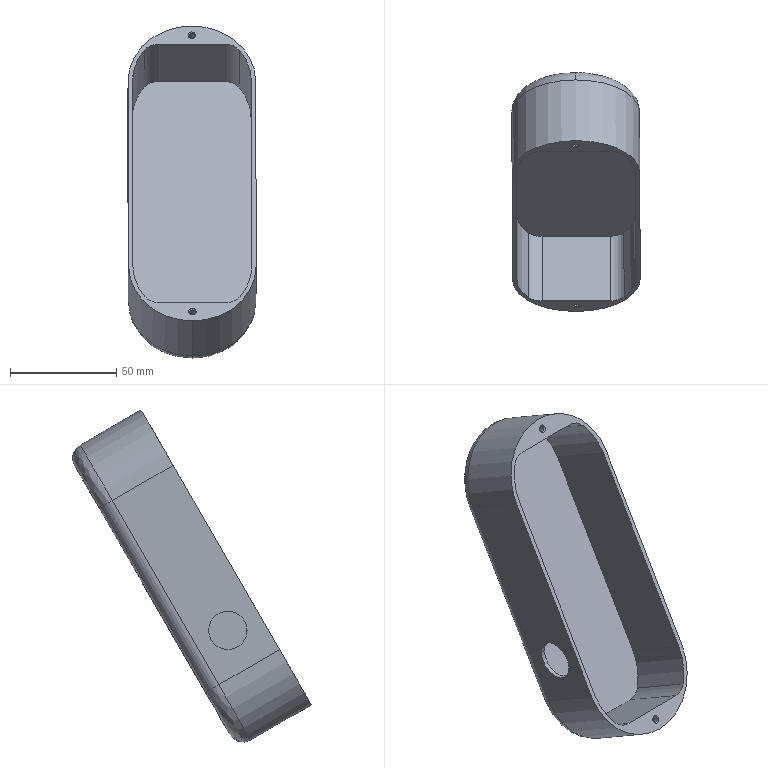Part | SolidWorks | features BaseBody 1 | 1 solid | 45 faces | box 60.342 x 112.079 x 156.002 mm | volume 81654 mm3 | cylinder 20 | plane 9 | spline 8 | cone 8 | commonest cylinder face diameters 16 x5 2.5 x4 56 x4 60 x3 14 x2 18 x2